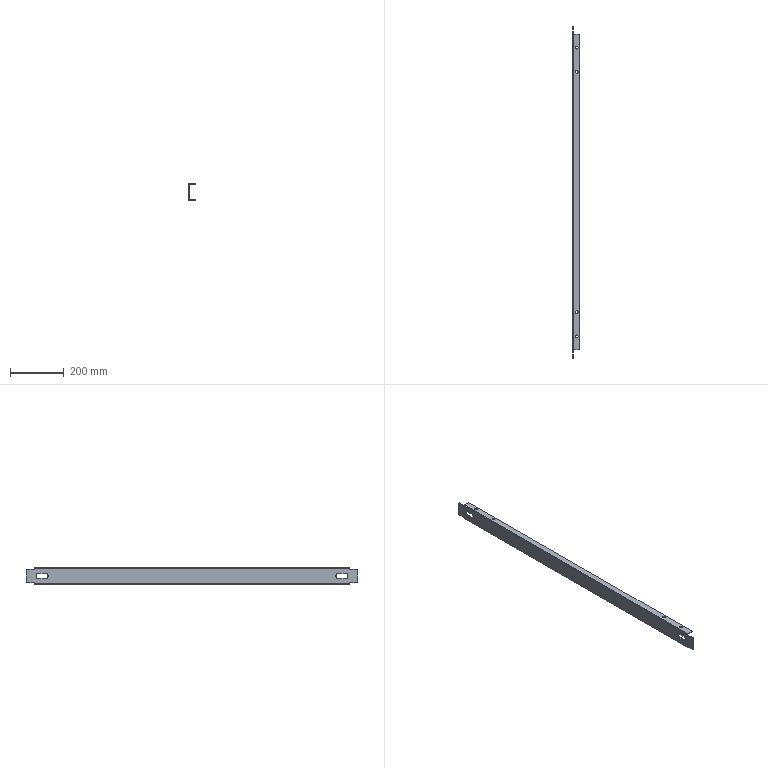Part | 1 solid | 58 faces | box 25 x 1239 x 62 mm | volume 371701 mm3 | plane 30 | cylinder 28 | commonest cylinder face diameters 11 x16 6 x4 20 x4 0.4 x2 6.4 x2